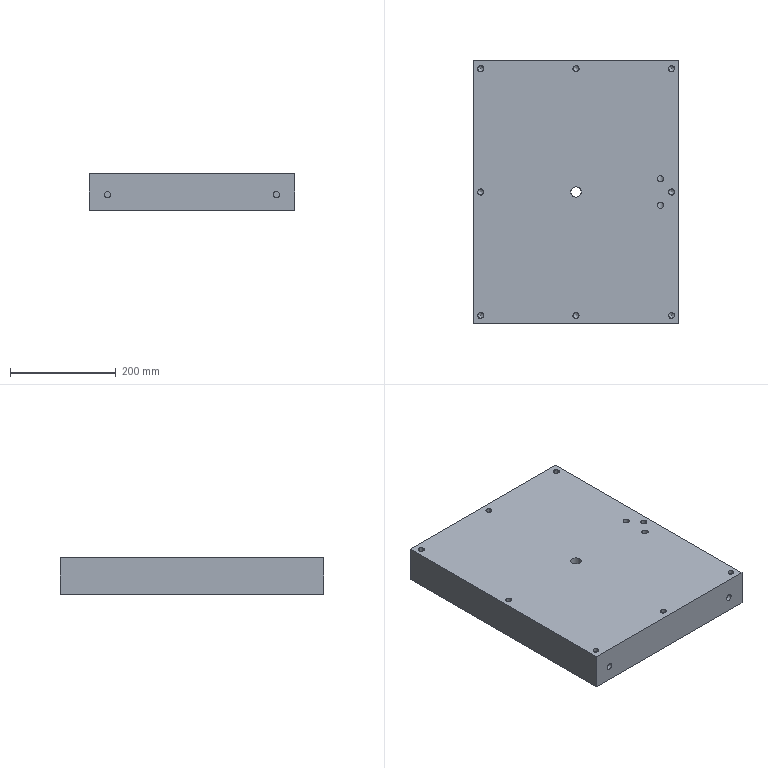Part | NX | features 模具.stp<1>[2] 2 | 1 solid | 151 faces | box 390 x 500 x 70 mm | volume 9093325 mm3 | plane 73 | cylinder 60 | sphere 10 | cone 8 | commonest cylinder face diameters 10 x20 12 x19 10.5 x8 11.7 x8 85 x2 91.927 x2